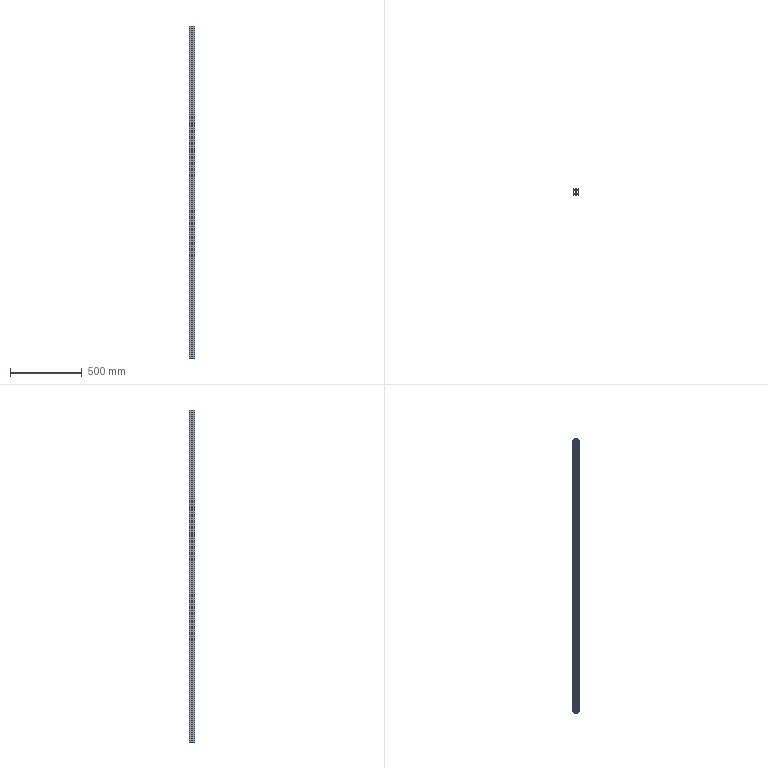Part | SolidWorks | features BaseBody 1, MoveFace 1 | 1 solid | 129 faces | box 40 x 40 x 2310 mm | volume 999614 mm3 | plane 102 | cylinder 27 | commonest cylinder face diameters 2 x8 1.5 x6 6.8 x5 6.6 x4 9 x4